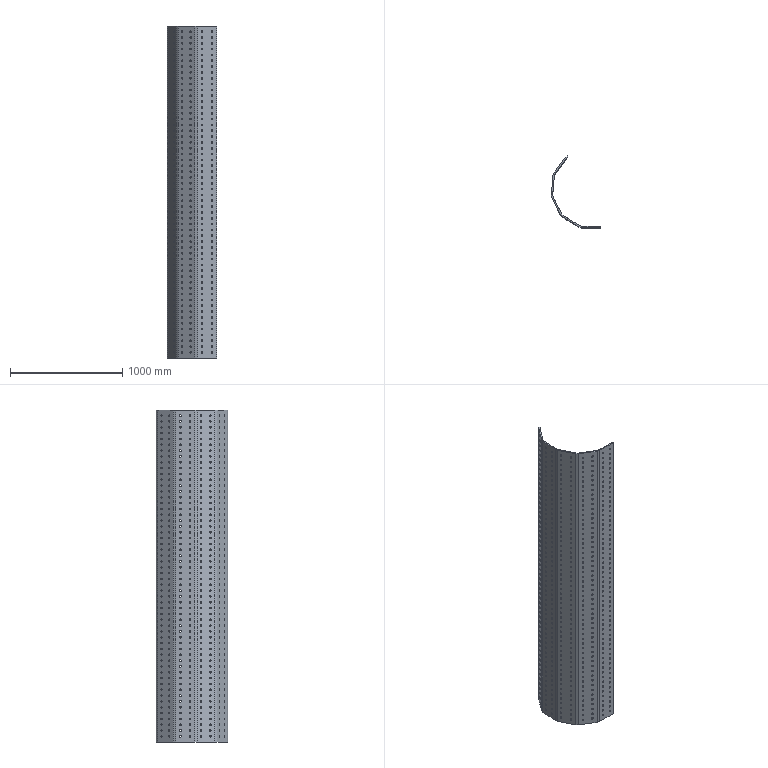Part | SolidWorks | features ICE 7, 3DProfileFeature 3, Extrusion 1 | 1 solid | 1144 faces | box 439.055 x 638.053 x 2960 mm | volume 32951018 mm3 | cylinder 1120 | plane 24 | commonest cylinder face diameters 15 x1120